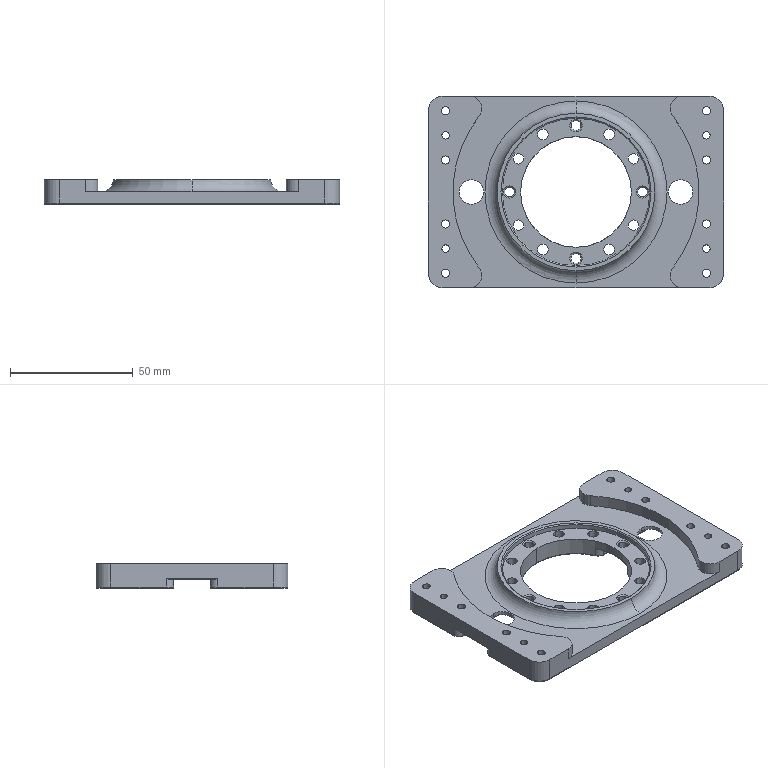NC program | NX | posted with a generic post | part box 120 x 78 x 10 mm
Lines 6065 to 6831 of 8419:
(ZLEVEL_PROFILE_1_COPY_1 , TOOL : D4R0.5)
N12110 T05 M6
N12112 G54
N12114 G17 G0 G90 X0.689 Y-34.785 B0. C0. S9500 M3
N12116 G43 Z30. H5
N12118 Z0.9
N12120 G94 G1 Z-0.1 F2500.
N12122 X0.346 Y-34.191
N12124 G3 X0. Y-33.991 R0.4
N12126 G2 X-33.991 Y0. R33.991
N12128 X0. Y-33.991 R-33.991
N12130 G1 X-0.136 Z-0.102
N12132 X-0.273 Y-33.989 Z-0.105
N12134 X-0.409 Y-33.988 Z-0.107
N12136 X-0.545 Y-33.987 Z-0.11
N12138 X-0.682 Y-33.985 Z-0.112
N12140 X-0.818 Y-33.982 Z-0.114
N12142 X-0.954 Y-33.978 Z-0.117
N12144 X-1.091 Y-33.974 Z-0.119
N12146 X-1.227 Y-33.97 Z-0.121
N12148 X-1.363 Y-33.965 Z-0.124
N12150 X-1.5 Y-33.958 Z-0.126
N12152 X-1.636 Y-33.952 Z-0.129
N12154 X-1.772 Y-33.945 Z-0.131
N12156 X-1.908 Y-33.939 Z-0.133
N12158 X-2.044 Y-33.93 Z-0.136
N12160 X-2.181 Y-33.921 Z-0.138
N12162 X-2.317 Y-33.912 Z-0.14
N12164 X-2.453 Y-33.903 Z-0.143
N12166 X-2.589 Y-33.894 Z-0.145
N12168 X-2.725 Y-33.883 Z-0.148
N12170 X-2.861 Y-33.871 Z-0.15
N12172 X-2.996 Y-33.859 Z-0.152
N12174 X-3.132 Y-33.848 Z-0.155
N12176 X-3.268 Y-33.835 Z-0.157
N12178 X-3.404 Y-33.821 Z-0.159
N12180 X-3.539 Y-33.807 Z-0.162
N12182 X-3.675 Y-33.793 Z-0.164
N12184 X-3.811 Y-33.778 Z-0.167
N12186 X-3.946 Y-33.763 Z-0.169
N12188 X-4.082 Y-33.747 Z-0.171
N12190 X-4.217 Y-33.731 Z-0.174
N12192 X-4.352 Y-33.713 Z-0.176
N12194 X-4.488 Y-33.696 Z-0.179
N12196 X-4.623 Y-33.677 Z-0.181
N12198 X-4.758 Y-33.658 Z-0.183
N12200 X-4.893 Y-33.638 Z-0.186
N12202 X-5.028 Y-33.619 Z-0.188
N12204 X-5.163 Y-33.599 Z-0.19
N12206 X-5.297 Y-33.578 Z-0.193
N12208 X-5.432 Y-33.556 Z-0.195
N12210 X-5.566 Y-33.534 Z-0.198
N12212 X-5.701 Y-33.512 Z-0.2
N12214 G2 X0. Y-33.993 R-33.993
N12216 G1 X-0.136 Z-0.202
N12218 X-0.273 Y-33.991 Z-0.205
N12220 X-0.409 Y-33.99 Z-0.207
N12222 X-0.545 Y-33.989 Z-0.209
N12224 X-0.682 Y-33.987 Z-0.212
N12226 X-0.818 Y-33.984 Z-0.214
N12228 X-0.954 Y-33.98 Z-0.217
N12230 X-1.091 Y-33.976 Z-0.219
N12232 X-1.227 Y-33.972 Z-0.221
N12234 X-1.363 Y-33.967 Z-0.224
N12236 X-1.5 Y-33.96 Z-0.226
N12238 X-1.636 Y-33.954 Z-0.229
N12240 X-1.772 Y-33.947 Z-0.231
N12242 X-1.908 Y-33.941 Z-0.233
N12244 X-2.044 Y-33.932 Z-0.236
N12246 X-2.181 Y-33.923 Z-0.238
N12248 X-2.317 Y-33.914 Z-0.24
N12250 X-2.453 Y-33.905 Z-0.243
N12252 X-2.589 Y-33.896 Z-0.245
N12254 X-2.725 Y-33.885 Z-0.248
N12256 X-2.861 Y-33.873 Z-0.25
N12258 X-2.996 Y-33.861 Z-0.252
N12260 X-3.132 Y-33.85 Z-0.255
N12262 X-3.268 Y-33.837 Z-0.257
N12264 X-3.404 Y-33.823 Z-0.259
N12266 X-3.539 Y-33.809 Z-0.262
N12268 X-3.675 Y-33.795 Z-0.264
N12270 X-3.811 Y-33.78 Z-0.267
N12272 X-3.946 Y-33.765 Z-0.269
N12274 X-4.082 Y-33.749 Z-0.271
N12276 X-4.217 Y-33.733 Z-0.274
N12278 X-4.352 Y-33.715 Z-0.276
N12280 X-4.488 Y-33.698 Z-0.279
N12282 X-4.623 Y-33.679 Z-0.281
N12284 X-4.758 Y-33.66 Z-0.283
N12286 X-4.893 Y-33.64 Z-0.286
N12288 X-5.028 Y-33.621 Z-0.288
N12290 X-5.163 Y-33.601 Z-0.29
N12292 X-5.297 Y-33.58 Z-0.293
N12294 X-5.432 Y-33.558 Z-0.295
N12296 X-5.566 Y-33.536 Z-0.298
N12298 X-5.701 Y-33.514 Z-0.3
N12300 G2 X0. Y-33.995 R-33.995
N12302 G1 X-0.136 Z-0.302
N12304 X-0.273 Y-33.994 Z-0.305
N12306 X-0.409 Y-33.992 Z-0.307
N12308 X-0.545 Y-33.991 Z-0.309
N12310 X-0.682 Y-33.989 Z-0.312
N12312 X-0.818 Y-33.986 Z-0.314
N12314 X-0.954 Y-33.982 Z-0.317
N12316 X-1.091 Y-33.978 Z-0.319
N12318 X-1.227 Y-33.974 Z-0.321
N12320 X-1.363 Y-33.969 Z-0.324
N12322 X-1.5 Y-33.962 Z-0.326
N12324 X-1.636 Y-33.956 Z-0.329
N12326 X-1.772 Y-33.949 Z-0.331
N12328 X-1.908 Y-33.943 Z-0.333
N12330 X-2.044 Y-33.935 Z-0.336
N12332 X-2.181 Y-33.925 Z-0.338
N12334 X-2.317 Y-33.916 Z-0.34
N12336 X-2.453 Y-33.907 Z-0.343
N12338 X-2.589 Y-33.898 Z-0.345
N12340 X-2.725 Y-33.887 Z-0.348
N12342 X-2.861 Y-33.875 Z-0.35
N12344 X-2.996 Y-33.863 Z-0.352
N12346 X-3.132 Y-33.852 Z-0.355
N12348 X-3.268 Y-33.84 Z-0.357
N12350 X-3.404 Y-33.825 Z-0.359
N12352 X-3.539 Y-33.811 Z-0.362
N12354 X-3.675 Y-33.797 Z-0.364
N12356 X-3.811 Y-33.782 Z-0.367
N12358 X-3.946 Y-33.767 Z-0.369
N12360 X-4.082 Y-33.751 Z-0.371
N12362 X-4.217 Y-33.735 Z-0.374
N12364 X-4.352 Y-33.717 Z-0.376
N12366 X-4.488 Y-33.7 Z-0.378
N12368 X-4.623 Y-33.681 Z-0.381
N12370 X-4.758 Y-33.662 Z-0.383
N12372 X-4.893 Y-33.642 Z-0.386
N12374 X-5.028 Y-33.623 Z-0.388
N12376 X-5.163 Y-33.603 Z-0.39
N12378 X-5.297 Y-33.582 Z-0.393
N12380 X-5.432 Y-33.56 Z-0.395
N12382 X-5.566 Y-33.538 Z-0.398
N12384 X-5.701 Y-33.516 Z-0.4
N12386 G2 X0. Y-33.998 R-33.998
N12388 G1 X-0.136 Y-33.997 Z-0.402
N12390 X-0.273 Y-33.996 Z-0.405
N12392 X-0.409 Y-33.994 Z-0.407
N12394 X-0.545 Y-33.993 Z-0.409
N12396 X-0.682 Y-33.991 Z-0.412
N12398 X-0.818 Y-33.988 Z-0.414
N12400 X-0.955 Y-33.984 Z-0.417
N12402 X-1.091 Y-33.98 Z-0.419
N12404 X-1.227 Y-33.976 Z-0.421
N12406 X-1.363 Y-33.971 Z-0.424
N12408 X-1.5 Y-33.961 Z-0.426
N12410 X-1.636 Y-33.955 Z-0.428
N12412 X-1.772 Y-33.949 Z-0.431
N12414 X-1.908 Y-33.945 Z-0.433
N12416 X-2.044 Y-33.934 Z-0.436
N12418 X-2.18 Y-33.926 Z-0.438
N12420 X-2.317 Y-33.917 Z-0.44
N12422 X-2.453 Y-33.908 Z-0.443
N12424 X-2.589 Y-33.9 Z-0.445
N12426 X-2.725 Y-33.888 Z-0.448
N12428 X-2.861 Y-33.877 Z-0.45
N12430 X-2.996 Y-33.865 Z-0.452
N12432 X-3.132 Y-33.853 Z-0.455
N12434 X-3.268 Y-33.842 Z-0.457
N12436 X-3.404 Y-33.828 Z-0.459
N12438 X-3.54 Y-33.814 Z-0.462
N12440 X-3.675 Y-33.799 Z-0.464
N12442 X-3.811 Y-33.785 Z-0.467
N12444 X-3.946 Y-33.77 Z-0.469
N12446 X-4.082 Y-33.753 Z-0.471
N12448 X-4.217 Y-33.737 Z-0.474
N12450 X-4.352 Y-33.72 Z-0.476
N12452 X-4.488 Y-33.702 Z-0.478
N12454 X-4.623 Y-33.684 Z-0.481
N12456 X-4.758 Y-33.665 Z-0.483
N12458 X-4.893 Y-33.646 Z-0.486
N12460 X-5.028 Y-33.626 Z-0.488
N12462 X-5.163 Y-33.606 Z-0.49
N12464 X-5.297 Y-33.585 Z-0.493
N12466 X-5.432 Y-33.563 Z-0.495
N12468 X-5.567 Y-33.541 Z-0.498
N12470 X-5.701 Y-33.519 Z-0.5
N12472 G2 X0. Y-34. R-34.
N12474 G1 X-0.136 Z-0.502
N12476 X-0.273 Y-33.999 Z-0.505
N12478 X-0.409 Y-33.998 Z-0.507
N12480 X-0.545 Y-33.996 Z-0.509
N12482 X-0.682 Y-33.994 Z-0.512
N12484 X-0.818 Y-33.991 Z-0.514
N12486 X-0.954 Y-33.987 Z-0.517
N12488 X-1.09 Y-33.983 Z-0.519
N12490 X-1.227 Y-33.979 Z-0.521
N12492 X-1.363 Y-33.973 Z-0.524
N12494 X-1.499 Y-33.968 Z-0.526
N12496 X-1.635 Y-33.961 Z-0.528
N12498 X-1.771 Y-33.955 Z-0.531
N12500 X-1.908 Y-33.947 Z-0.533
N12502 X-2.044 Y-33.94 Z-0.536
N12504 X-2.18 Y-33.931 Z-0.538
N12506 X-2.316 Y-33.922 Z-0.54
N12508 X-2.452 Y-33.913 Z-0.543
N12510 X-2.588 Y-33.903 Z-0.545
N12512 X-2.724 Y-33.892 Z-0.547
N12514 X-2.859 Y-33.881 Z-0.55
N12516 X-2.995 Y-33.869 Z-0.552
N12518 X-3.131 Y-33.857 Z-0.555
N12520 X-3.267 Y-33.844 Z-0.557
N12522 X-3.402 Y-33.831 Z-0.559
N12524 X-3.538 Y-33.817 Z-0.562
N12526 X-3.674 Y-33.803 Z-0.564
N12528 X-3.809 Y-33.788 Z-0.567
N12530 X-3.945 Y-33.773 Z-0.569
N12532 X-4.08 Y-33.757 Z-0.571
N12534 X-4.215 Y-33.74 Z-0.574
N12536 X-4.351 Y-33.723 Z-0.576
N12538 X-4.486 Y-33.705 Z-0.578
N12540 X-4.621 Y-33.687 Z-0.581
N12542 X-4.756 Y-33.668 Z-0.583
N12544 X-4.891 Y-33.649 Z-0.586
N12546 X-5.026 Y-33.629 Z-0.588
N12548 X-5.161 Y-33.609 Z-0.59
N12550 X-5.295 Y-33.588 Z-0.593
N12552 X-5.43 Y-33.567 Z-0.595
N12554 X-5.565 Y-33.545 Z-0.597
N12556 X-5.699 Y-33.522 Z-0.6
N12558 G2 X0. Y-34.003 R-34.003
N12560 G1 X-0.136 Z-0.602
N12562 X-0.272 Z-0.605
N12564 X-0.409 Y-34.001 Z-0.607
N12566 X-0.545 Y-34. Z-0.609
N12568 X-0.681 Y-33.997 Z-0.612
N12570 X-0.817 Y-33.994 Z-0.614
N12572 X-0.953 Y-33.991 Z-0.616
N12574 X-1.089 Y-33.987 Z-0.619
N12576 X-1.225 Y-33.982 Z-0.621
N12578 X-1.361 Y-33.977 Z-0.624
N12580 X-1.498 Y-33.972 Z-0.626
N12582 X-1.634 Y-33.966 Z-0.628
N12584 X-1.77 Y-33.959 Z-0.631
N12586 X-1.906 Y-33.952 Z-0.633
N12588 X-2.042 Y-33.944 Z-0.635
N12590 X-2.178 Y-33.936 Z-0.638
N12592 X-2.313 Y-33.927 Z-0.64
N12594 X-2.449 Y-33.917 Z-0.643
N12596 X-2.585 Y-33.907 Z-0.645
N12598 X-2.721 Y-33.897 Z-0.647
N12600 X-2.857 Y-33.886 Z-0.65
N12602 X-2.992 Y-33.874 Z-0.652
N12604 X-3.128 Y-33.862 Z-0.655
N12606 X-3.264 Y-33.849 Z-0.657
N12608 X-3.399 Y-33.836 Z-0.659
N12610 X-3.535 Y-33.822 Z-0.662
N12612 X-3.67 Y-33.808 Z-0.664
N12614 X-3.805 Y-33.793 Z-0.666
N12616 X-3.941 Y-33.778 Z-0.669
N12618 X-4.076 Y-33.762 Z-0.671
N12620 X-4.211 Y-33.746 Z-0.674
N12622 X-4.346 Y-33.729 Z-0.676
N12624 X-4.481 Y-33.711 Z-0.678
N12626 X-4.616 Y-33.693 Z-0.681
N12628 X-4.751 Y-33.674 Z-0.683
N12630 X-4.886 Y-33.655 Z-0.685
N12632 X-5.021 Y-33.636 Z-0.688
N12634 X-5.156 Y-33.615 Z-0.69
N12636 X-5.29 Y-33.595 Z-0.693
N12638 X-5.425 Y-33.573 Z-0.695
N12640 X-5.559 Y-33.551 Z-0.697
N12642 X-5.694 Y-33.529 Z-0.7
N12644 G2 X0. Y-34.009 R-34.009
N12646 G1 X-0.136 Z-0.702
N12648 X-0.272 Y-34.008 Z-0.704
N12650 X-0.408 Y-34.007 Z-0.707
N12652 X-0.544 Y-34.005 Z-0.709
N12654 X-0.68 Y-34.003 Z-0.712
N12656 X-0.816 Y-34. Z-0.714
N12658 X-0.952 Y-33.997 Z-0.716
N12660 X-1.088 Y-33.993 Z-0.719
N12662 X-1.224 Y-33.988 Z-0.721
N12664 X-1.359 Y-33.983 Z-0.723
N12666 X-1.495 Y-33.978 Z-0.726
N12668 X-1.631 Y-33.972 Z-0.728
N12670 X-1.767 Y-33.965 Z-0.731
N12672 X-1.903 Y-33.958 Z-0.733
N12674 X-2.039 Y-33.95 Z-0.735
N12676 X-2.174 Y-33.942 Z-0.738
N12678 X-2.31 Y-33.933 Z-0.74
N12680 X-2.446 Y-33.924 Z-0.742
N12682 X-2.581 Y-33.914 Z-0.745
N12684 X-2.717 Y-33.904 Z-0.747
N12686 X-2.852 Y-33.893 Z-0.75
N12688 X-2.988 Y-33.881 Z-0.752
N12690 X-3.123 Y-33.869 Z-0.754
N12692 X-3.259 Y-33.857 Z-0.757
N12694 X-3.394 Y-33.844 Z-0.759
N12696 X-3.53 Y-33.83 Z-0.761
N12698 X-3.665 Y-33.816 Z-0.764
N12700 X-3.8 Y-33.801 Z-0.766
N12702 X-3.935 Y-33.786 Z-0.769
N12704 X-4.07 Y-33.77 Z-0.771
N12706 X-4.205 Y-33.754 Z-0.773
N12708 X-4.34 Y-33.737 Z-0.776
N12710 X-4.475 Y-33.719 Z-0.778
N12712 X-4.61 Y-33.701 Z-0.78
N12714 X-4.745 Y-33.683 Z-0.783
N12716 X-4.879 Y-33.664 Z-0.785
N12718 X-5.014 Y-33.644 Z-0.787
N12720 X-5.148 Y-33.624 Z-0.79
N12722 X-5.283 Y-33.603 Z-0.792
N12724 X-5.417 Y-33.582 Z-0.795
N12726 X-5.551 Y-33.561 Z-0.797
N12728 X-5.686 Y-33.538 Z-0.799
N12730 G2 X0. Y-34.017 R-34.017
N12732 G1 X-0.136 Z-0.802
N12734 X-0.271 Y-34.016 Z-0.804
N12736 X-0.407 Y-34.015 Z-0.806
N12738 X-0.543 Y-34.013 Z-0.809
N12740 X-0.678 Y-34.011 Z-0.811
N12742 X-0.814 Y-34.008 Z-0.814
N12744 X-0.95 Y-34.005 Z-0.816
N12746 X-1.085 Y-34.001 Z-0.818
N12748 X-1.221 Y-33.997 Z-0.821
N12750 X-1.357 Y-33.992 Z-0.823
N12752 X-1.492 Y-33.986 Z-0.825
N12754 X-1.628 Y-33.98 Z-0.828
N12756 X-1.764 Y-33.974 Z-0.83
N12758 X-1.899 Y-33.967 Z-0.833
N12760 X-2.035 Y-33.959 Z-0.835
N12762 X-2.17 Y-33.951 Z-0.837
N12764 X-2.305 Y-33.942 Z-0.84
N12766 X-2.441 Y-33.933 Z-0.842
N12768 X-2.576 Y-33.923 Z-0.844
N12770 X-2.712 Y-33.913 Z-0.847
N12772 X-2.847 Y-33.902 Z-0.849
N12774 X-2.982 Y-33.891 Z-0.851
N12776 X-3.117 Y-33.879 Z-0.854
N12778 X-3.252 Y-33.866 Z-0.856
N12780 X-3.388 Y-33.853 Z-0.859
N12782 X-3.523 Y-33.84 Z-0.861
N12784 X-3.658 Y-33.826 Z-0.863
N12786 X-3.793 Y-33.811 Z-0.866
N12788 X-3.927 Y-33.796 Z-0.868
N12790 X-4.062 Y-33.78 Z-0.87
N12792 X-4.197 Y-33.764 Z-0.873
N12794 X-4.332 Y-33.747 Z-0.875
N12796 X-4.466 Y-33.73 Z-0.878
N12798 X-4.601 Y-33.712 Z-0.88
N12800 X-4.735 Y-33.694 Z-0.882
N12802 X-4.87 Y-33.675 Z-0.885
N12804 X-5.004 Y-33.655 Z-0.887
N12806 X-5.138 Y-33.635 Z-0.889
N12808 X-5.273 Y-33.615 Z-0.892
N12810 X-5.407 Y-33.594 Z-0.894
N12812 X-5.541 Y-33.572 Z-0.896
N12814 X-5.675 Y-33.55 Z-0.899
N12816 G2 X0. Y-34.027 R-34.027
N12818 G1 X-0.135 Z-0.901
N12820 X-0.271 Y-34.026 Z-0.904
N12822 X-0.406 Y-34.025 Z-0.906
N12824 X-0.541 Y-34.023 Z-0.908
N12826 X-0.677 Y-34.021 Z-0.911
N12828 X-0.812 Y-34.019 Z-0.913
N12830 X-0.947 Y-34.015 Z-0.915
N12832 X-1.083 Y-34.012 Z-0.918
N12834 X-1.218 Y-34.007 Z-0.92
N12836 X-1.353 Y-34.003 Z-0.922
N12838 X-1.489 Y-33.997 Z-0.925
N12840 X-1.624 Y-33.991 Z-0.927
N12842 X-1.759 Y-33.985 Z-0.93
N12844 X-1.894 Y-33.978 Z-0.932
N12846 X-2.03 Y-33.97 Z-0.934
N12848 X-2.165 Y-33.962 Z-0.937
N12850 X-2.3 Y-33.954 Z-0.939
N12852 X-2.435 Y-33.944 Z-0.941
N12854 X-2.57 Y-33.935 Z-0.944
N12856 X-2.705 Y-33.925 Z-0.946
N12858 X-2.84 Y-33.914 Z-0.948
N12860 X-2.975 Y-33.903 Z-0.951
N12862 X-3.11 Y-33.891 Z-0.953
N12864 X-3.244 Y-33.878 Z-0.956
N12866 X-3.379 Y-33.866 Z-0.958
N12868 X-3.514 Y-33.852 Z-0.96
N12870 X-3.649 Y-33.838 Z-0.963
N12872 X-3.783 Y-33.824 Z-0.965
N12874 X-3.918 Y-33.809 Z-0.967
N12876 X-4.052 Y-33.793 Z-0.97
N12878 X-4.187 Y-33.777 Z-0.972
N12880 X-4.321 Y-33.76 Z-0.974
N12882 X-4.455 Y-33.743 Z-0.977
N12884 X-4.59 Y-33.726 Z-0.979
N12886 X-4.724 Y-33.707 Z-0.982
N12888 X-4.858 Y-33.689 Z-0.984
N12890 X-4.992 Y-33.669 Z-0.986
N12892 X-5.126 Y-33.649 Z-0.989
N12894 X-5.26 Y-33.629 Z-0.991
N12896 X-5.394 Y-33.608 Z-0.993
N12898 X-5.527 Y-33.587 Z-0.996
N12900 X-5.661 Y-33.565 Z-0.998
N12902 G2 X0. Y-34.039 R-34.039
N12904 G1 X-0.135 Z-1.
N12906 X-0.27 Y-34.038 Z-1.003
N12908 X-0.405 Y-34.037 Z-1.005
N12910 X-0.54 Y-34.036 Z-1.008
N12912 X-0.675 Y-34.034 Z-1.01
N12914 X-0.81 Y-34.031 Z-1.012
N12916 X-0.945 Y-34.028 Z-1.015
N12918 X-1.08 Y-34.024 Z-1.017
N12920 X-1.214 Y-34.02 Z-1.019
N12922 X-1.349 Y-34.015 Z-1.022
N12924 X-1.484 Y-34.01 Z-1.024
N12926 X-1.619 Y-34.004 Z-1.026
N12928 X-1.754 Y-33.998 Z-1.029
N12930 X-1.889 Y-33.991 Z-1.031
N12932 X-2.023 Y-33.984 Z-1.033
N12934 X-2.158 Y-33.976 Z-1.036
N12936 X-2.293 Y-33.967 Z-1.038
N12938 X-2.428 Y-33.958 Z-1.04
N12940 X-2.562 Y-33.949 Z-1.043
N12942 X-2.697 Y-33.939 Z-1.045
N12944 X-2.831 Y-33.928 Z-1.048
N12946 X-2.966 Y-33.917 Z-1.05
N12948 X-3.1 Y-33.905 Z-1.052
N12950 X-3.235 Y-33.893 Z-1.055
N12952 X-3.369 Y-33.88 Z-1.057
N12954 X-3.504 Y-33.867 Z-1.059
N12956 X-3.638 Y-33.853 Z-1.062
N12958 X-3.772 Y-33.839 Z-1.064
N12960 X-3.906 Y-33.824 Z-1.066
N12962 X-4.04 Y-33.808 Z-1.069
N12964 X-4.174 Y-33.792 Z-1.071
N12966 X-4.308 Y-33.776 Z-1.073
N12968 X-4.442 Y-33.759 Z-1.076
N12970 X-4.576 Y-33.741 Z-1.078
N12972 X-4.71 Y-33.723 Z-1.081
N12974 X-4.844 Y-33.705 Z-1.083
N12976 X-4.977 Y-33.686 Z-1.085
N12978 X-5.111 Y-33.666 Z-1.088
N12980 X-5.244 Y-33.646 Z-1.09
N12982 X-5.378 Y-33.625 Z-1.092
N12984 X-5.511 Y-33.604 Z-1.095
N12986 X-5.644 Y-33.582 Z-1.097
N12988 G2 X0. Y-34.053 R-34.053
N12990 G1 X-0.141 Z-1.099
N12992 X-0.282 Z-1.102
N12994 X-0.424 Y-34.052 Z-1.104
N12996 X-0.565 Y-34.05 Z-1.107
N12998 X-0.706 Y-34.048 Z-1.109
N13000 X-0.847 Y-34.045 Z-1.112
N13002 X-0.988 Y-34.042 Z-1.114
N13004 X-1.13 Y-34.038 Z-1.117
N13006 X-1.271 Y-34.033 Z-1.119
N13008 X-1.412 Y-34.028 Z-1.122
N13010 X-1.553 Y-34.022 Z-1.124
N13012 X-1.694 Y-34.016 Z-1.127
N13014 X-1.835 Y-34.009 Z-1.129
N13016 X-1.976 Y-34.001 Z-1.132
N13018 X-2.117 Y-33.993 Z-1.134
N13020 X-2.258 Y-33.985 Z-1.136
N13022 X-2.399 Y-33.975 Z-1.139
N13024 X-2.54 Y-33.966 Z-1.141
N13026 X-2.681 Y-33.955 Z-1.144
N13028 X-2.822 Y-33.944 Z-1.146
N13030 X-2.962 Y-33.933 Z-1.149
N13032 X-3.103 Y-33.921 Z-1.151
N13034 X-3.244 Y-33.908 Z-1.154
N13036 X-3.384 Y-33.894 Z-1.156
N13038 X-3.525 Y-33.881 Z-1.159
N13040 X-3.665 Y-33.866 Z-1.161
N13042 X-3.806 Y-33.851 Z-1.164
N13044 X-3.946 Y-33.835 Z-1.166
N13046 X-4.087 Y-33.819 Z-1.169
N13048 X-4.227 Y-33.802 Z-1.171
N13050 X-4.367 Y-33.785 Z-1.173
N13052 X-4.507 Y-33.767 Z-1.176
N13054 X-4.647 Y-33.748 Z-1.178
N13056 X-4.787 Y-33.729 Z-1.181
N13058 X-4.927 Y-33.71 Z-1.183
N13060 X-5.067 Y-33.689 Z-1.186
N13062 X-5.207 Y-33.668 Z-1.188
N13064 X-5.346 Y-33.647 Z-1.191
N13066 X-5.486 Y-33.625 Z-1.193
N13068 X-5.625 Y-33.602 Z-1.196
N13070 G2 X0. Y-34.07 R-34.07
N13072 G1 X-0.141 Z-1.198
N13074 X-0.281 Z-1.201
N13076 X-0.422 Y-34.069 Z-1.203
N13078 X-0.563 Y-34.067 Z-1.205
N13080 X-0.703 Y-34.065 Z-1.208
N13082 X-0.844 Y-34.062 Z-1.21
N13084 X-0.984 Y-34.059 Z-1.213
N13086 X-1.125 Y-34.055 Z-1.215
N13088 X-1.266 Y-34.05 Z-1.218
N13090 X-1.406 Y-34.045 Z-1.22
N13092 X-1.547 Y-34.04 Z-1.223
N13094 X-1.687 Y-34.033 Z-1.225
N13096 X-1.828 Y-34.027 Z-1.228
N13098 X-1.968 Y-34.019 Z-1.23
N13100 X-2.109 Y-34.011 Z-1.232
N13102 X-2.249 Y-34.003 Z-1.235
N13104 X-2.39 Y-33.994 Z-1.237
N13106 X-2.53 Y-33.984 Z-1.24
N13108 X-2.67 Y-33.974 Z-1.242
N13110 X-2.81 Y-33.963 Z-1.245
N13112 X-2.951 Y-33.951 Z-1.247
N13114 X-3.091 Y-33.939 Z-1.25
N13116 X-3.231 Y-33.927 Z-1.252
N13118 X-3.371 Y-33.914 Z-1.255
N13120 X-3.511 Y-33.9 Z-1.257
N13122 X-3.651 Y-33.886 Z-1.259
N13124 X-3.791 Y-33.871 Z-1.262
N13126 X-3.931 Y-33.855 Z-1.264
N13128 X-4.071 Y-33.839 Z-1.267
N13130 X-4.21 Y-33.823 Z-1.269
N13132 X-4.35 Y-33.806 Z-1.272
N13134 X-4.489 Y-33.788 Z-1.274
N13136 X-4.629 Y-33.769 Z-1.277
N13138 X-4.768 Y-33.751 Z-1.279
N13140 X-4.908 Y-33.731 Z-1.282
N13142 X-5.047 Y-33.711 Z-1.284
N13144 X-5.186 Y-33.69 Z-1.286
N13146 X-5.325 Y-33.669 Z-1.289
N13148 X-5.464 Y-33.647 Z-1.291
N13150 X-5.603 Y-33.625 Z-1.294
N13152 G2 X0. Y-34.089 R-34.089
N13154 G1 X-0.14 Z-1.296
N13156 X-0.28 Z-1.299
N13158 X-0.42 Y-34.088 Z-1.301
N13160 X-0.56 Y-34.086 Z-1.304
N13162 X-0.7 Y-34.084 Z-1.306
N13164 X-0.84 Y-34.081 Z-1.308
N13166 X-0.98 Y-34.078 Z-1.311
N13168 X-1.12 Y-34.074 Z-1.313
N13170 X-1.26 Y-34.07 Z-1.316
N13172 X-1.4 Y-34.065 Z-1.318
N13174 X-1.54 Y-34.059 Z-1.321
N13176 X-1.68 Y-34.053 Z-1.323
N13178 X-1.82 Y-34.047 Z-1.326
N13180 X-1.959 Y-34.039 Z-1.328
N13182 X-2.099 Y-34.032 Z-1.33
N13184 X-2.239 Y-34.023 Z-1.333
N13186 X-2.379 Y-34.014 Z-1.335
N13188 X-2.519 Y-34.005 Z-1.338
N13190 X-2.658 Y-33.995 Z-1.34
N13192 X-2.798 Y-33.984 Z-1.343
N13194 X-2.937 Y-33.973 Z-1.345
N13196 X-3.077 Y-33.961 Z-1.348
N13198 X-3.217 Y-33.948 Z-1.35
N13200 X-3.356 Y-33.935 Z-1.352
N13202 X-3.495 Y-33.922 Z-1.355
N13204 X-3.635 Y-33.908 Z-1.357
N13206 X-3.774 Y-33.893 Z-1.36
N13208 X-3.913 Y-33.878 Z-1.362
N13210 X-4.052 Y-33.862 Z-1.365
N13212 X-4.192 Y-33.846 Z-1.367
N13214 X-4.331 Y-33.829 Z-1.37
N13216 X-4.47 Y-33.811 Z-1.372
N13218 X-4.608 Y-33.793 Z-1.374
N13220 X-4.747 Y-33.774 Z-1.377
N13222 X-4.886 Y-33.755 Z-1.379
N13224 X-5.025 Y-33.735 Z-1.382
N13226 X-5.163 Y-33.715 Z-1.384
N13228 X-5.302 Y-33.694 Z-1.387
N13230 X-5.44 Y-33.672 Z-1.389
N13232 X-5.579 Y-33.65 Z-1.392
N13234 G2 X0. Y-34.11 R-34.11
N13236 G1 X-0.139 Z-1.394
N13238 X-0.279 Z-1.396
N13240 X-0.418 Y-34.109 Z-1.399
N13242 X-0.557 Y-34.107 Z-1.401
N13244 X-0.697 Y-34.105 Z-1.404
N13246 X-0.836 Y-34.103 Z-1.406
N13248 X-0.975 Y-34.1 Z-1.409
N13250 X-1.114 Y-34.096 Z-1.411
N13252 X-1.254 Y-34.092 Z-1.413
N13254 X-1.393 Y-34.087 Z-1.416
N13256 X-1.532 Y-34.081 Z-1.418
N13258 X-1.671 Y-34.075 Z-1.421
N13260 X-1.81 Y-34.069 Z-1.423
N13262 X-1.95 Y-34.062 Z-1.426
N13264 X-2.089 Y-34.054 Z-1.428
N13266 X-2.228 Y-34.046 Z-1.43
N13268 X-2.367 Y-34.037 Z-1.433
N13270 X-2.506 Y-34.028 Z-1.435
N13272 X-2.645 Y-34.018 Z-1.438
N13274 X-2.784 Y-34.007 Z-1.44
N13276 X-2.923 Y-33.996 Z-1.443
N13278 X-3.062 Y-33.984 Z-1.445
N13280 X-3.2 Y-33.972 Z-1.448
N13282 X-3.339 Y-33.959 Z-1.45
N13284 X-3.478 Y-33.946 Z-1.452
N13286 X-3.617 Y-33.932 Z-1.455
N13288 X-3.755 Y-33.918 Z-1.457
N13290 X-3.894 Y-33.903 Z-1.46
N13292 X-4.032 Y-33.887 Z-1.462
N13294 X-4.171 Y-33.871 Z-1.465
N13296 X-4.309 Y-33.854 Z-1.467
N13298 X-4.447 Y-33.837 Z-1.469
N13300 X-4.586 Y-33.819 Z-1.472
N13302 X-4.724 Y-33.801 Z-1.474
N13304 X-4.862 Y-33.782 Z-1.477
N13306 X-5. Y-33.762 Z-1.479
N13308 X-5.138 Y-33.742 Z-1.482
N13310 X-5.276 Y-33.721 Z-1.484
N13312 X-5.413 Y-33.7 Z-1.486
N13314 X-5.551 Y-33.678 Z-1.489
N13316 G2 X0. Y-34.133 R-34.133
N13318 G1 X-0.139 Z-1.491
N13320 X-0.277 Z-1.494
N13322 X-0.416 Y-34.132 Z-1.496
N13324 X-0.554 Y-34.131 Z-1.499
N13326 X-0.693 Y-34.129 Z-1.501
N13328 X-0.831 Y-34.126 Z-1.503
N13330 X-0.97 Y-34.123 Z-1.506
N13332 X-1.108 Y-34.12 Z-1.508
N13334 X-1.247 Y-34.115 Z-1.511
N13336 X-1.385 Y-34.111 Z-1.513
N13338 X-1.524 Y-34.105 Z-1.515
N13340 X-1.662 Y-34.1 Z-1.518
N13342 X-1.8 Y-34.093 Z-1.52
N13344 X-1.939 Y-34.086 Z-1.523
N13346 X-2.077 Y-34.079 Z-1.525
N13348 X-2.216 Y-34.071 Z-1.528
N13350 X-2.354 Y-34.062 Z-1.53
N13352 X-2.492 Y-34.053 Z-1.532
N13354 X-2.63 Y-34.043 Z-1.535
N13356 X-2.769 Y-34.033 Z-1.537
N13358 X-2.907 Y-34.022 Z-1.54
N13360 X-3.045 Y-34.01 Z-1.542
N13362 X-3.183 Y-33.998 Z-1.544
N13364 X-3.321 Y-33.986 Z-1.547
N13366 X-3.459 Y-33.973 Z-1.549
N13368 X-3.597 Y-33.959 Z-1.552
N13370 X-3.735 Y-33.945 Z-1.554
N13372 X-3.872 Y-33.93 Z-1.557
N13374 X-4.01 Y-33.915 Z-1.559
N13376 X-4.148 Y-33.899 Z-1.561
N13378 X-4.286 Y-33.882 Z-1.564
N13380 X-4.423 Y-33.865 Z-1.566
N13382 X-4.561 Y-33.848 Z-1.569
N13384 X-4.698 Y-33.829 Z-1.571
N13386 X-4.835 Y-33.811 Z-1.573
N13388 X-4.973 Y-33.791 Z-1.576
N13390 X-5.11 Y-33.772 Z-1.578
N13392 X-5.247 Y-33.751 Z-1.581
N13394 X-5.384 Y-33.73 Z-1.583
N13396 X-5.521 Y-33.709 Z-1.586
N13398 G2 X0. Y-34.158 R-34.158
N13400 G1 X-0.138 Z-1.588
N13402 X-0.275 Z-1.59
N13404 X-0.413 Y-34.157 Z-1.593
N13406 X-0.551 Y-34.156 Z-1.595
N13408 X-0.688 Y-34.154 Z-1.598
N13410 X-0.826 Y-34.152 Z-1.6
N13412 X-0.964 Y-34.149 Z-1.602
N13414 X-1.101 Y-34.146 Z-1.605
N13416 X-1.239 Y-34.141 Z-1.607
N13418 X-1.377 Y-34.137 Z-1.61
N13420 X-1.514 Y-34.132 Z-1.612
N13422 X-1.652 Y-34.126 Z-1.614
N13424 X-1.79 Y-34.12 Z-1.617
N13426 X-1.927 Y-34.113 Z-1.619
N13428 X-2.065 Y-34.106 Z-1.622
N13430 X-2.202 Y-34.098 Z-1.624
N13432 X-2.34 Y-34.089 Z-1.626
N13434 X-2.477 Y-34.08 Z-1.629
N13436 X-2.614 Y-34.071 Z-1.631
N13438 X-2.752 Y-34.06 Z-1.634
N13440 X-2.889 Y-34.05 Z-1.636
N13442 X-3.026 Y-34.038 Z-1.638
N13444 X-3.164 Y-34.027 Z-1.641
N13446 X-3.301 Y-34.014 Z-1.643
N13448 X-3.438 Y-34.001 Z-1.646
N13450 X-3.575 Y-33.988 Z-1.648
N13452 X-3.712 Y-33.974 Z-1.65
N13454 X-3.849 Y-33.959 Z-1.653
N13456 X-3.986 Y-33.944 Z-1.655
N13458 X-4.123 Y-33.929 Z-1.658
N13460 X-4.26 Y-33.913 Z-1.66
N13462 X-4.397 Y-33.896 Z-1.662
N13464 X-4.533 Y-33.878 Z-1.665
N13466 X-4.67 Y-33.861 Z-1.667
N13468 X-4.806 Y-33.842 Z-1.67
N13470 X-4.943 Y-33.823 Z-1.672
N13472 X-5.079 Y-33.804 Z-1.674
N13474 X-5.216 Y-33.784 Z-1.677
N13476 X-5.352 Y-33.763 Z-1.679
N13478 X-5.488 Y-33.742 Z-1.682
N13480 G2 X0. Y-34.185 R-34.185
N13482 G1 X-0.137 Y-34.186 Z-1.684
N13484 X-0.274 Z-1.686
N13486 X-0.41 Y-34.185 Z-1.689
N13488 X-0.547 Y-34.184 Z-1.691
N13490 X-0.684 Y-34.182 Z-1.694
N13492 X-0.821 Y-34.18 Z-1.696
N13494 X-0.957 Y-34.177 Z-1.698
N13496 X-1.094 Y-34.174 Z-1.701
N13498 X-1.231 Y-34.17 Z-1.703
N13500 X-1.368 Y-34.165 Z-1.706
N13502 X-1.504 Y-34.16 Z-1.708
N13504 X-1.641 Y-34.155 Z-1.71
N13506 X-1.778 Y-34.148 Z-1.713
N13508 X-1.914 Y-34.142 Z-1.715
N13510 X-2.051 Y-34.135 Z-1.718
N13512 X-2.188 Y-34.127 Z-1.72
N13514 X-2.324 Y-34.119 Z-1.722
N13516 X-2.461 Y-34.11 Z-1.725
N13518 X-2.597 Y-34.1 Z-1.727
N13520 X-2.734 Y-34.09 Z-1.729
N13522 X-2.87 Y-34.08 Z-1.732
N13524 X-3.007 Y-34.069 Z-1.734
N13526 X-3.143 Y-34.057 Z-1.737
N13528 X-3.279 Y-34.045 Z-1.739
N13530 X-3.416 Y-34.033 Z-1.741
N13532 X-3.552 Y-34.019 Z-1.744
N13534 X-3.688 Y-34.006 Z-1.746
N13536 X-3.824 Y-33.991 Z-1.749
N13538 X-3.96 Y-33.977 Z-1.751
N13540 X-4.096 Y-33.961 Z-1.753
N13542 X-4.232 Y-33.945 Z-1.756
N13544 X-4.368 Y-33.929 Z-1.758
N13546 X-4.504 Y-33.912 Z-1.76
N13548 X-4.64 Y-33.894 Z-1.763
N13550 X-4.775 Y-33.876 Z-1.765
N13552 X-4.911 Y-33.858 Z-1.768
N13554 X-5.046 Y-33.838 Z-1.77
N13556 X-5.182 Y-33.819 Z-1.772
N13558 X-5.317 Y-33.798 Z-1.775
N13560 X-5.453 Y-33.778 Z-1.777
N13562 G2 X0. Y-34.215 R-34.215
N13564 G1 X-0.136 Z-1.78
N13566 X-0.272 Z-1.782
N13568 X-0.407 Z-1.784
N13570 X-0.543 Y-34.214 Z-1.787
N13572 X-0.679 Y-34.212 Z-1.789
N13574 X-0.815 Y-34.21 Z-1.791
N13576 X-0.951 Y-34.207 Z-1.794
N13578 X-1.086 Y-34.204 Z-1.796
N13580 X-1.222 Y-34.2 Z-1.799
N13582 X-1.358 Y-34.196 Z-1.801
N13584 X-1.494 Y-34.191 Z-1.803
N13586 X-1.629 Y-34.185 Z-1.806
N13588 X-1.765 Y-34.179 Z-1.808
N13590 X-1.901 Y-34.173 Z-1.81
N13592 X-2.036 Y-34.166 Z-1.813
N13594 X-2.172 Y-34.158 Z-1.815
N13596 X-2.308 Y-34.15 Z-1.817
N13598 X-2.443 Y-34.142 Z-1.82
N13600 X-2.579 Y-34.132 Z-1.822
N13602 X-2.714 Y-34.123 Z-1.825
N13604 X-2.85 Y-34.112 Z-1.827
N13606 X-2.985 Y-34.102 Z-1.829
N13608 X-3.121 Y-34.09 Z-1.832
N13610 X-3.256 Y-34.078 Z-1.834
N13612 X-3.391 Y-34.066 Z-1.836
N13614 X-3.527 Y-34.053 Z-1.839
N13616 X-3.662 Y-34.04 Z-1.841
N13618 X-3.797 Y-34.026 Z-1.844
N13620 X-3.932 Y-34.011 Z-1.846
N13622 X-4.067 Y-33.996 Z-1.848
N13624 X-4.202 Y-33.98 Z-1.851
N13626 X-4.337 Y-33.964 Z-1.853
N13628 X-4.472 Y-33.948 Z-1.855
N13630 X-4.607 Y-33.93 Z-1.858
N13632 X-4.741 Y-33.913 Z-1.86
N13634 X-4.876 Y-33.894 Z-1.863
N13636 X-5.011 Y-33.876 Z-1.865